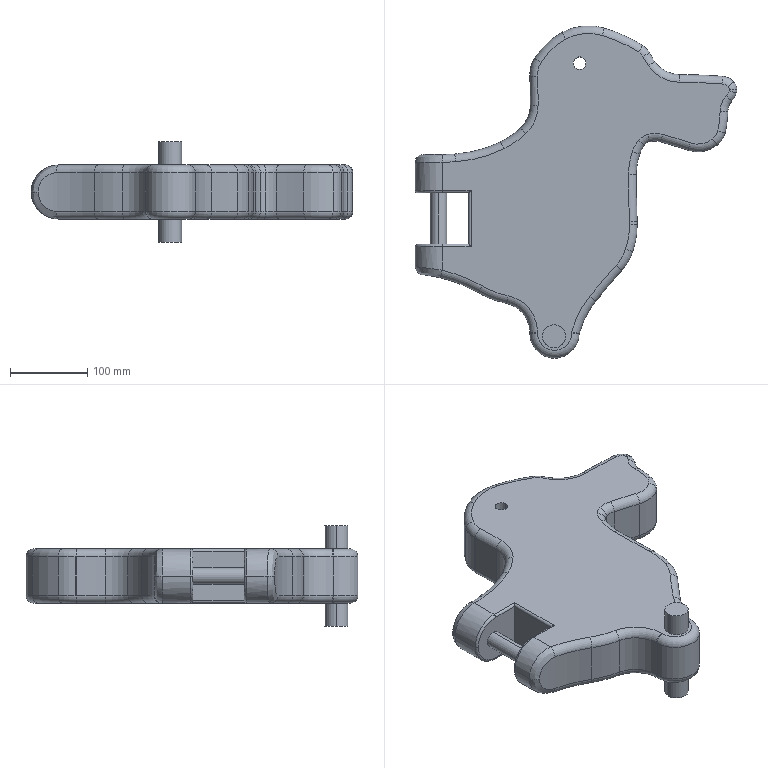Part | SolidWorks | features ICE 4, Fillet 3 | 1 solid | 144 faces | box 416.464 x 430.21 x 130 mm | volume 5952307 mm3 | torus 80 | cylinder 53 | plane 7 | spline 4 | commonest cylinder face diameters 6 x6 29.974 x4 70 x4 16.263 x2 21.397 x2 83.393 x2